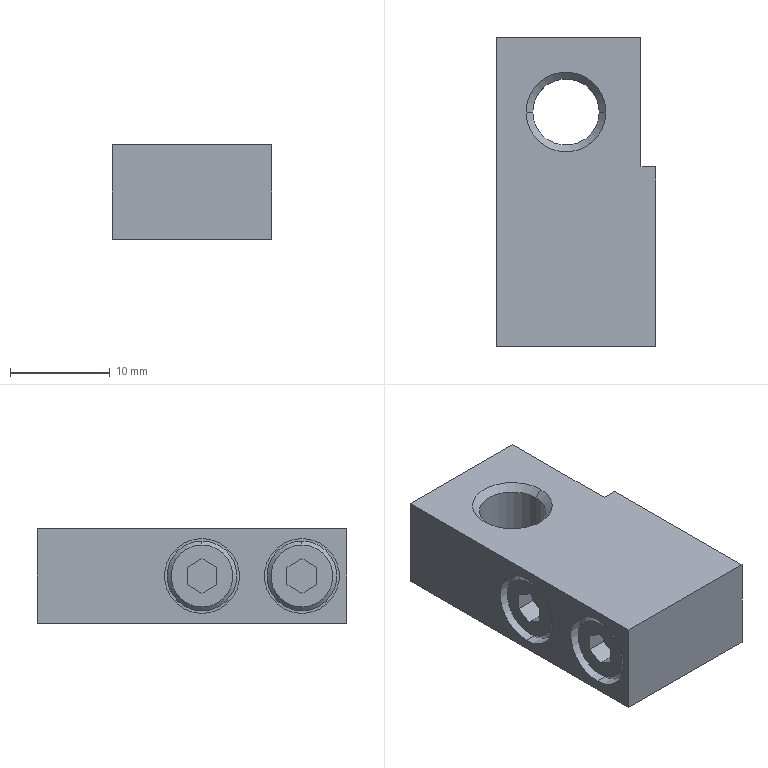Part | SolidWorks | features BaseBody 1 | 1 solid | 44 faces | box 16 x 31 x 9.5 mm | volume 4071 mm3 | plane 26 | cylinder 10 | cone 8 | commonest cylinder face diameters 7 x4 7.5 x4 6.647 x2
STEP:
#1=CARTESIAN_POINT('',(-15.6,4.5,3.1));
#2=VERTEX_POINT('',#1);
#3=CARTESIAN_POINT('',(-15.6,4.5,-3.1));
#4=VERTEX_POINT('',#3);
#5=CARTESIAN_POINT('',(-15.6,4.5,0.));
#6=DIRECTION('',(-1.,0.,0.));
#7=DIRECTION('',(0.,0.,1.));
#8=AXIS2_PLACEMENT_3D('',#5,#6,#7);
#9=CIRCLE('',#8,3.1);
#10=EDGE_CURVE('',#2,#4,#9,.T.);
#11=ORIENTED_EDGE('',*,*,#10,.F.);
#12=CARTESIAN_POINT('',(-15.2,4.5,3.5));
#13=VERTEX_POINT('',#12);
#14=CARTESIAN_POINT('',(-15.2,4.5,3.5));
#15=DIRECTION('',(0.7071,0.,0.7071));
#16=VECTOR('',#15,1000.);
#17=LINE('',#14,#16);
#18=EDGE_CURVE('',#2,#13,#17,.T.);
#19=ORIENTED_EDGE('',*,*,#18,.T.);
#20=CARTESIAN_POINT('',(-15.2,4.5,-3.5));
#21=VERTEX_POINT('',#20);
#22=CARTESIAN_POINT('',(-15.2,4.5,0.));
#23=DIRECTION('',(-1.,0.,0.));
#24=DIRECTION('',(0.,0.,1.));
#25=AXIS2_PLACEMENT_3D('',#22,#23,#24);
#26=CIRCLE('',#25,3.5);
#27=EDGE_CURVE('',#13,#21,#26,.T.);
#28=ORIENTED_EDGE('',*,*,#27,.T.);
#29=CARTESIAN_POINT('',(-15.2,4.5,-3.5));
#30=DIRECTION('',(0.7071,0.,-0.7071));
#31=VECTOR('',#30,1000.);
#32=LINE('',#29,#31);
#33=EDGE_CURVE('',#4,#21,#32,.T.);
#34=ORIENTED_EDGE('',*,*,#33,.F.);
#35=EDGE_LOOP('',(#11,#19,#28,#34));
#36=FACE_OUTER_BOUND('',#35,.T.);
#37=CARTESIAN_POINT('',(-15.2,4.5,0.));
#38=DIRECTION('',(1.,0.,0.));
#39=DIRECTION('',(0.,0.,-1.));
#40=AXIS2_PLACEMENT_3D('',#37,#38,#39);
#41=CONICAL_SURFACE('',#40,3.5,0.7854);
#42=ADVANCED_FACE('',(#36),#41,.T.);
#43=CARTESIAN_POINT('',(-5.677,23.5,4.074));
#44=VERTEX_POINT('',#43);
#45=CARTESIAN_POINT('',(-12.324,23.5,4.074));
#46=VERTEX_POINT('',#45);
#47=CARTESIAN_POINT('',(-9.,23.5,4.074));
#48=DIRECTION('',(0.,0.,-1.));
#49=DIRECTION('',(-1.,0.,0.));
#50=AXIS2_PLACEMENT_3D('',#47,#48,#49);
#51=CIRCLE('',#50,3.324);
#52=EDGE_CURVE('',#44,#46,#51,.T.);
#53=ORIENTED_EDGE('',*,*,#52,.F.);
#54=CARTESIAN_POINT('',(-5.677,23.5,-4.074));
#55=VERTEX_POINT('',#54);
#56=CARTESIAN_POINT('',(-5.677,23.5,-4.75));
#57=DIRECTION('',(0.,0.,-1.));
#58=VECTOR('',#57,1000.);
#59=LINE('',#56,#58);
#60=EDGE_CURVE('',#44,#55,#59,.T.);
#61=ORIENTED_EDGE('',*,*,#60,.T.);
#62=CARTESIAN_POINT('',(-12.324,23.5,-4.074));
#63=VERTEX_POINT('',#62);
#64=CARTESIAN_POINT('',(-9.,23.5,-4.074));
#65=DIRECTION('',(0.,0.,-1.));
#66=DIRECTION('',(-1.,0.,0.));
#67=AXIS2_PLACEMENT_3D('',#64,#65,#66);
#68=CIRCLE('',#67,3.324);
#69=EDGE_CURVE('',#55,#63,#68,.T.);
#70=ORIENTED_EDGE('',*,*,#69,.T.);
#71=CARTESIAN_POINT('',(-12.324,23.5,-4.75));
#72=DIRECTION('',(0.,0.,-1.));
#73=VECTOR('',#72,1000.);
#74=LINE('',#71,#73);
#75=EDGE_CURVE('',#46,#63,#74,.T.);
#76=ORIENTED_EDGE('',*,*,#75,.F.);
#77=EDGE_LOOP('',(#53,#61,#70,#76));
#78=FACE_OUTER_BOUND('',#77,.T.);
#79=CARTESIAN_POINT('',(-9.,23.5,-4.75));
#80=DIRECTION('',(0.,0.,-1.));
#81=DIRECTION('',(-1.,0.,0.));
#82=AXIS2_PLACEMENT_3D('',#79,#80,#81);
#83=CYLINDRICAL_SURFACE('',#82,3.324);
#84=ADVANCED_FACE('',(#78),#83,.F.);
#85=CARTESIAN_POINT('',(-11.6,4.5,3.5));
#86=VERTEX_POINT('',#85);
#87=CARTESIAN_POINT('',(-11.6,4.5,-3.5));
#88=VERTEX_POINT('',#87);
#89=CARTESIAN_POINT('',(-11.6,4.5,0.));
#90=DIRECTION('',(-1.,0.,0.));
#91=DIRECTION('',(0.,0.,-1.));
#92=AXIS2_PLACEMENT_3D('',#89,#90,#91);
#93=CIRCLE('',#92,3.5);
#94=EDGE_CURVE('',#86,#88,#93,.T.);
#95=ORIENTED_EDGE('',*,*,#94,.T.);
#96=CARTESIAN_POINT('',(-15.6,4.5,-3.5));
#97=DIRECTION('',(-1.,0.,0.));
#98=VECTOR('',#97,1000.);
#99=LINE('',#96,#98);
#100=EDGE_CURVE('',#88,#21,#99,.T.);
#101=ORIENTED_EDGE('',*,*,#100,.T.);
#102=ORIENTED_EDGE('',*,*,#27,.F.);
#103=CARTESIAN_POINT('',(-15.6,4.5,3.5));
#104=DIRECTION('',(-1.,0.,0.));
#105=VECTOR('',#104,1000.);
#106=LINE('',#103,#105);
#107=EDGE_CURVE('',#86,#13,#106,.T.);
#108=ORIENTED_EDGE('',*,*,#107,.F.);
#109=EDGE_LOOP('',(#95,#101,#102,#108));
#110=FACE_OUTER_BOUND('',#109,.T.);
#111=CARTESIAN_POINT('',(-15.6,4.5,0.));
#112=DIRECTION('',(-1.,0.,0.));
#113=DIRECTION('',(0.,0.,1.));
#114=AXIS2_PLACEMENT_3D('',#111,#112,#113);
#115=CYLINDRICAL_SURFACE('',#114,3.5);
#116=ADVANCED_FACE('',(#110),#115,.T.);
#117=ORIENTED_EDGE('',*,*,#52,.T.);
#118=CARTESIAN_POINT('',(-13.,23.5,4.75));
#119=VERTEX_POINT('',#118);
#120=CARTESIAN_POINT('',(-13.,23.5,4.75));
#121=DIRECTION('',(-0.7071,0.,0.7071));
#122=VECTOR('',#121,1000.);
#123=LINE('',#120,#122);
#124=EDGE_CURVE('',#46,#119,#123,.T.);
#125=ORIENTED_EDGE('',*,*,#124,.T.);
#126=CARTESIAN_POINT('',(-5.,23.5,4.75));
#127=VERTEX_POINT('',#126);
#128=CARTESIAN_POINT('',(-9.,23.5,4.75));
#129=DIRECTION('',(0.,0.,-1.));
#130=DIRECTION('',(-1.,0.,0.));
#131=AXIS2_PLACEMENT_3D('',#128,#129,#130);
#132=CIRCLE('',#131,4.);
#133=EDGE_CURVE('',#127,#119,#132,.T.);
#134=ORIENTED_EDGE('',*,*,#133,.F.);
#135=CARTESIAN_POINT('',(-5.,23.5,4.75));
#136=DIRECTION('',(0.7071,0.,0.7071));
#137=VECTOR('',#136,1000.);
#138=LINE('',#135,#137);
#139=EDGE_CURVE('',#44,#127,#138,.T.);
#140=ORIENTED_EDGE('',*,*,#139,.F.);
#141=EDGE_LOOP('',(#117,#125,#134,#140));
#142=FACE_OUTER_BOUND('',#141,.T.);
#143=CARTESIAN_POINT('',(-9.,23.5,4.75));
#144=DIRECTION('',(0.,0.,1.));
#145=DIRECTION('',(1.,0.,0.));
#146=AXIS2_PLACEMENT_3D('',#143,#144,#145);
#147=CONICAL_SURFACE('',#146,4.,0.7854);
#148=ADVANCED_FACE('',(#142),#147,.F.);
#149=ORIENTED_EDGE('',*,*,#69,.F.);
#150=CARTESIAN_POINT('',(-5.,23.5,-4.75));
#151=VERTEX_POINT('',#150);
#152=CARTESIAN_POINT('',(-5.677,23.5,-4.074));
#153=DIRECTION('',(0.7071,0.,-0.7071));
#154=VECTOR('',#153,1000.);
#155=LINE('',#152,#154);
#156=EDGE_CURVE('',#55,#151,#155,.T.);
#157=ORIENTED_EDGE('',*,*,#156,.T.);
#158=CARTESIAN_POINT('',(-13.,23.5,-4.75));
#159=VERTEX_POINT('',#158);
#160=CARTESIAN_POINT('',(-9.,23.5,-4.75));
#161=DIRECTION('',(0.,0.,-1.));
#162=DIRECTION('',(-1.,0.,0.));
#163=AXIS2_PLACEMENT_3D('',#160,#161,#162);
#164=CIRCLE('',#163,4.);
#165=EDGE_CURVE('',#151,#159,#164,.T.);
#166=ORIENTED_EDGE('',*,*,#165,.T.);
#167=CARTESIAN_POINT('',(-12.324,23.5,-4.074));
#168=DIRECTION('',(-0.7071,0.,-0.7071));
#169=VECTOR('',#168,1000.);
#170=LINE('',#167,#169);
#171=EDGE_CURVE('',#63,#159,#170,.T.);
#172=ORIENTED_EDGE('',*,*,#171,.F.);
#173=EDGE_LOOP('',(#149,#157,#166,#172));
#174=FACE_OUTER_BOUND('',#173,.T.);
#175=CARTESIAN_POINT('',(-9.,23.5,-4.074));
#176=DIRECTION('',(0.,0.,-1.));
#177=DIRECTION('',(-1.,0.,0.));
#178=AXIS2_PLACEMENT_3D('',#175,#176,#177);
#179=CONICAL_SURFACE('',#178,3.324,0.7854);
#180=ADVANCED_FACE('',(#174),#179,.F.);
#181=CARTESIAN_POINT('',(-11.6,4.5,3.75));
#182=VERTEX_POINT('',#181);
#183=CARTESIAN_POINT('',(-11.6,4.5,-3.75));
#184=VERTEX_POINT('',#183);
#185=CARTESIAN_POINT('',(-11.6,4.5,0.));
#186=DIRECTION('',(1.,0.,0.));
#187=DIRECTION('',(0.,0.,-1.));
#188=AXIS2_PLACEMENT_3D('',#185,#186,#187);
#189=CIRCLE('',#188,3.75);
#190=EDGE_CURVE('',#182,#184,#189,.T.);
#191=ORIENTED_EDGE('',*,*,#190,.T.);
#192=CARTESIAN_POINT('',(-16.,4.5,-3.75));
#193=VERTEX_POINT('',#192);
#194=CARTESIAN_POINT('',(-11.6,4.5,-3.75));
#195=DIRECTION('',(-1.,0.,0.));
#196=VECTOR('',#195,1000.);
#197=LINE('',#194,#196);
#198=EDGE_CURVE('',#184,#193,#197,.T.);
#199=ORIENTED_EDGE('',*,*,#198,.T.);
#200=CARTESIAN_POINT('',(-16.,4.5,3.75));
#201=VERTEX_POINT('',#200);
#202=CARTESIAN_POINT('',(-16.,4.5,0.));
#203=DIRECTION('',(1.,0.,0.));
#204=DIRECTION('',(0.,0.,-1.));
#205=AXIS2_PLACEMENT_3D('',#202,#203,#204);
#206=CIRCLE('',#205,3.75);
#207=EDGE_CURVE('',#201,#193,#206,.T.);
#208=ORIENTED_EDGE('',*,*,#207,.F.);
#209=CARTESIAN_POINT('',(-11.6,4.5,3.75));
#210=DIRECTION('',(-1.,0.,0.));
#211=VECTOR('',#210,1000.);
#212=LINE('',#209,#211);
#213=EDGE_CURVE('',#182,#201,#212,.T.);
#214=ORIENTED_EDGE('',*,*,#213,.F.);
#215=EDGE_LOOP('',(#191,#199,#208,#214));
#216=FACE_OUTER_BOUND('',#215,.T.);
#217=CARTESIAN_POINT('',(-11.6,4.5,0.));
#218=DIRECTION('',(-1.,0.,0.));
#219=DIRECTION('',(0.,0.,1.));
#220=AXIS2_PLACEMENT_3D('',#217,#218,#219);
#221=CYLINDRICAL_SURFACE('',#220,3.75);
#222=ADVANCED_FACE('',(#216),#221,.F.);
#223=CARTESIAN_POINT('',(-11.6,14.5,3.75));
#224=VERTEX_POINT('',#223);
#225=CARTESIAN_POINT('',(-11.6,14.5,-3.75));
#226=VERTEX_POINT('',#225);
#227=CARTESIAN_POINT('',(-11.6,14.5,0.));
#228=DIRECTION('',(1.,0.,0.));
#229=DIRECTION('',(0.,0.,-1.));
#230=AXIS2_PLACEMENT_3D('',#227,#228,#229);
#231=CIRCLE('',#230,3.75);
#232=EDGE_CURVE('',#224,#226,#231,.T.);
#233=ORIENTED_EDGE('',*,*,#232,.T.);
#234=CARTESIAN_POINT('',(-16.,14.5,-3.75));
#235=VERTEX_POINT('',#234);
#236=CARTESIAN_POINT('',(-11.6,14.5,-3.75));
#237=DIRECTION('',(-1.,0.,0.));
#238=VECTOR('',#237,1000.);
#239=LINE('',#236,#238);
#240=EDGE_CURVE('',#226,#235,#239,.T.);
#241=ORIENTED_EDGE('',*,*,#240,.T.);
#242=CARTESIAN_POINT('',(-16.,14.5,3.75));
#243=VERTEX_POINT('',#242);
#244=CARTESIAN_POINT('',(-16.,14.5,0.));
#245=DIRECTION('',(1.,0.,0.));
#246=DIRECTION('',(0.,0.,-1.));
#247=AXIS2_PLACEMENT_3D('',#244,#245,#246);
#248=CIRCLE('',#247,3.75);
#249=EDGE_CURVE('',#243,#235,#248,.T.);
#250=ORIENTED_EDGE('',*,*,#249,.F.);
#251=CARTESIAN_POINT('',(-11.6,14.5,3.75));
#252=DIRECTION('',(-1.,0.,0.));
#253=VECTOR('',#252,1000.);
#254=LINE('',#251,#253);
#255=EDGE_CURVE('',#224,#243,#254,.T.);
#256=ORIENTED_EDGE('',*,*,#255,.F.);
#257=EDGE_LOOP('',(#233,#241,#250,#256));
#258=FACE_OUTER_BOUND('',#257,.T.);
#259=CARTESIAN_POINT('',(-11.6,14.5,0.));
#260=DIRECTION('',(-1.,0.,0.));
#261=DIRECTION('',(0.,0.,1.));
#262=AXIS2_PLACEMENT_3D('',#259,#260,#261);
#263=CYLINDRICAL_SURFACE('',#262,3.75);
#264=ADVANCED_FACE('',(#258),#263,.F.);
#265=CARTESIAN_POINT('',(-11.6,14.5,3.5));
#266=VERTEX_POINT('',#265);
#267=CARTESIAN_POINT('',(-11.6,14.5,-3.5));
#268=VERTEX_POINT('',#267);
#269=CARTESIAN_POINT('',(-11.6,14.5,0.));
#270=DIRECTION('',(-1.,0.,0.));
#271=DIRECTION('',(0.,0.,-1.));
#272=AXIS2_PLACEMENT_3D('',#269,#270,#271);
#273=CIRCLE('',#272,3.5);
#274=EDGE_CURVE('',#266,#268,#273,.T.);
#275=ORIENTED_EDGE('',*,*,#274,.T.);
#276=CARTESIAN_POINT('',(-15.2,14.5,-3.5));
#277=VERTEX_POINT('',#276);
#278=CARTESIAN_POINT('',(-15.6,14.5,-3.5));
#279=DIRECTION('',(-1.,0.,0.));
#280=VECTOR('',#279,1000.);
#281=LINE('',#278,#280);
#282=EDGE_CURVE('',#268,#277,#281,.T.);
#283=ORIENTED_EDGE('',*,*,#282,.T.);
#284=CARTESIAN_POINT('',(-15.2,14.5,3.5));
#285=VERTEX_POINT('',#284);
#286=CARTESIAN_POINT('',(-15.2,14.5,0.));
#287=DIRECTION('',(-1.,0.,0.));
#288=DIRECTION('',(0.,0.,1.));
#289=AXIS2_PLACEMENT_3D('',#286,#287,#288);
#290=CIRCLE('',#289,3.5);
#291=EDGE_CURVE('',#285,#277,#290,.T.);
#292=ORIENTED_EDGE('',*,*,#291,.F.);
#293=CARTESIAN_POINT('',(-15.6,14.5,3.5));
#294=DIRECTION('',(-1.,0.,0.));
#295=VECTOR('',#294,1000.);
#296=LINE('',#293,#295);
#297=EDGE_CURVE('',#266,#285,#296,.T.);
#298=ORIENTED_EDGE('',*,*,#297,.F.);
#299=EDGE_LOOP('',(#275,#283,#292,#298));
#300=FACE_OUTER_BOUND('',#299,.T.);
#301=CARTESIAN_POINT('',(-15.6,14.5,0.));
#302=DIRECTION('',(-1.,0.,0.));
#303=DIRECTION('',(0.,0.,1.));
#304=AXIS2_PLACEMENT_3D('',#301,#302,#303);
#305=CYLINDRICAL_SURFACE('',#304,3.5);
#306=ADVANCED_FACE('',(#300),#305,.T.);
#307=CARTESIAN_POINT('',(-15.6,14.5,3.1));
#308=VERTEX_POINT('',#307);
#309=CARTESIAN_POINT('',(-15.6,14.5,-3.1));
#310=VERTEX_POINT('',#309);
#311=CARTESIAN_POINT('',(-15.6,14.5,0.));
#312=DIRECTION('',(-1.,0.,0.));
#313=DIRECTION('',(0.,0.,1.));
#314=AXIS2_PLACEMENT_3D('',#311,#312,#313);
#315=CIRCLE('',#314,3.1);
#316=EDGE_CURVE('',#308,#310,#315,.T.);
#317=ORIENTED_EDGE('',*,*,#316,.F.);
#318=CARTESIAN_POINT('',(-15.2,14.5,3.5));
#319=DIRECTION('',(0.7071,0.,0.7071));
#320=VECTOR('',#319,1000.);
#321=LINE('',#318,#320);
#322=EDGE_CURVE('',#308,#285,#321,.T.);
#323=ORIENTED_EDGE('',*,*,#322,.T.);
#324=ORIENTED_EDGE('',*,*,#291,.T.);
#325=CARTESIAN_POINT('',(-15.2,14.5,-3.5));
#326=DIRECTION('',(0.7071,0.,-0.7071));
#327=VECTOR('',#326,1000.);
#328=LINE('',#325,#327);
#329=EDGE_CURVE('',#310,#277,#328,.T.);
#330=ORIENTED_EDGE('',*,*,#329,.F.);
#331=EDGE_LOOP('',(#317,#323,#324,#330));
#332=FACE_OUTER_BOUND('',#331,.T.);
#333=CARTESIAN_POINT('',(-15.2,14.5,0.));
#334=DIRECTION('',(1.,0.,0.));
#335=DIRECTION('',(0.,0.,-1.));
#336=AXIS2_PLACEMENT_3D('',#333,#334,#335);
#337=CONICAL_SURFACE('',#336,3.5,0.7854);
#338=ADVANCED_FACE('',(#332),#337,.T.);
#339=CARTESIAN_POINT('',(-15.6,14.5,1.732));
#340=VERTEX_POINT('',#339);
#341=CARTESIAN_POINT('',(-15.6,13.,0.866));
#342=VERTEX_POINT('',#341);
#343=CARTESIAN_POINT('',(-15.6,14.5,1.732));
#344=DIRECTION('',(0.,-0.866,-0.5));
#345=VECTOR('',#344,1000.);
#346=LINE('',#343,#345);
#347=EDGE_CURVE('',#340,#342,#346,.T.);
#348=ORIENTED_EDGE('',*,*,#347,.T.);
#349=CARTESIAN_POINT('',(-15.6,13.,-0.866));
#350=VERTEX_POINT('',#349);
#351=CARTESIAN_POINT('',(-15.6,13.,-0.866));
#352=DIRECTION('',(0.,0.,1.));
#353=VECTOR('',#352,1000.);
#354=LINE('',#351,#353);
#355=EDGE_CURVE('',#350,#342,#354,.T.);
#356=ORIENTED_EDGE('',*,*,#355,.F.);
#357=CARTESIAN_POINT('',(-15.6,14.5,-1.732));
#358=VERTEX_POINT('',#357);
#359=CARTESIAN_POINT('',(-15.6,13.,-0.866));
#360=DIRECTION('',(0.,0.866,-0.5));
#361=VECTOR('',#360,1000.);
#362=LINE('',#359,#361);
#363=EDGE_CURVE('',#350,#358,#362,.T.);
#364=ORIENTED_EDGE('',*,*,#363,.T.);
#365=CARTESIAN_POINT('',(-15.6,16.,-0.866));
#366=VERTEX_POINT('',#365);
#367=CARTESIAN_POINT('',(-15.6,14.5,-1.732));
#368=DIRECTION('',(0.,0.866,0.5));
#369=VECTOR('',#368,1000.);
#370=LINE('',#367,#369);
#371=EDGE_CURVE('',#358,#366,#370,.T.);
#372=ORIENTED_EDGE('',*,*,#371,.T.);
#373=CARTESIAN_POINT('',(-15.6,16.,0.866));
#374=VERTEX_POINT('',#373);
#375=CARTESIAN_POINT('',(-15.6,16.,-0.866));
#376=DIRECTION('',(0.,0.,1.));
#377=VECTOR('',#376,1000.);
#378=LINE('',#375,#377);
#379=EDGE_CURVE('',#366,#374,#378,.T.);
#380=ORIENTED_EDGE('',*,*,#379,.T.);
#381=CARTESIAN_POINT('',(-15.6,16.,0.866));
#382=DIRECTION('',(0.,-0.866,0.5));
#383=VECTOR('',#382,1000.);
#384=LINE('',#381,#383);
#385=EDGE_CURVE('',#374,#340,#384,.T.);
#386=ORIENTED_EDGE('',*,*,#385,.T.);
#387=EDGE_LOOP('',(#348,#356,#364,#372,#380,#386));
#388=FACE_BOUND('',#387,.T.);
#389=CARTESIAN_POINT('',(-15.6,14.5,0.));
#390=DIRECTION('',(-1.,0.,0.));
#391=DIRECTION('',(0.,0.,1.));
#392=AXIS2_PLACEMENT_3D('',#389,#390,#391);
#393=CIRCLE('',#392,3.1);
#394=EDGE_CURVE('',#310,#308,#393,.T.);
#395=ORIENTED_EDGE('',*,*,#394,.T.);
#396=ORIENTED_EDGE('',*,*,#316,.T.);
#397=EDGE_LOOP('',(#395,#396));
#398=FACE_OUTER_BOUND('',#397,.T.);
#399=CARTESIAN_POINT('',(-15.6,11.4,0.));
#400=DIRECTION('',(1.,0.,0.));
#401=DIRECTION('',(0.,0.,-1.));
#402=AXIS2_PLACEMENT_3D('',#399,#400,#401);
#403=PLANE('',#402);
#404=ADVANCED_FACE('',(#388,#398),#403,.F.);
#405=ORIENTED_EDGE('',*,*,#347,.F.);
#406=CARTESIAN_POINT('',(-13.6,14.5,1.732));
#407=VERTEX_POINT('',#406);
#408=CARTESIAN_POINT('',(-13.6,14.5,1.732));
#409=DIRECTION('',(-1.,0.,0.));
#410=VECTOR('',#409,1000.);
#411=LINE('',#408,#410);
#412=EDGE_CURVE('',#407,#340,#411,.T.);
#413=ORIENTED_EDGE('',*,*,#412,.F.);
#414=CARTESIAN_POINT('',(-13.6,13.,0.866));
#415=VERTEX_POINT('',#414);
#416=CARTESIAN_POINT('',(-13.6,14.5,1.732));
#417=DIRECTION('',(0.,-0.866,-0.5));
#418=VECTOR('',#417,1000.);
#419=LINE('',#416,#418);
#420=EDGE_CURVE('',#407,#415,#419,.T.);
#421=ORIENTED_EDGE('',*,*,#420,.T.);
#422=CARTESIAN_POINT('',(-13.6,13.,0.866));
#423=DIRECTION('',(-1.,0.,0.));
#424=VECTOR('',#423,1000.);
#425=LINE('',#422,#424);
#426=EDGE_CURVE('',#415,#342,#425,.T.);
#427=ORIENTED_EDGE('',*,*,#426,.T.);
#428=EDGE_LOOP('',(#405,#413,#421,#427));
#429=FACE_OUTER_BOUND('',#428,.T.);
#430=CARTESIAN_POINT('',(-13.6,14.5,1.732));
#431=DIRECTION('',(0.,0.5,-0.866));
#432=DIRECTION('',(0.,0.866,0.5));
#433=AXIS2_PLACEMENT_3D('',#430,#431,#432);
#434=PLANE('',#433);
#435=ADVANCED_FACE('',(#429),#434,.T.);
#436=ORIENTED_EDGE('',*,*,#355,.T.);
#437=ORIENTED_EDGE('',*,*,#426,.F.);
#438=CARTESIAN_POINT('',(-13.6,13.,-0.866));
#439=VERTEX_POINT('',#438);
#440=CARTESIAN_POINT('',(-13.6,13.,0.866));
#441=DIRECTION('',(0.,0.,-1.));
#442=VECTOR('',#441,1000.);
#443=LINE('',#440,#442);
#444=EDGE_CURVE('',#415,#439,#443,.T.);
#445=ORIENTED_EDGE('',*,*,#444,.T.);
#446=CARTESIAN_POINT('',(-13.6,13.,-0.866));
#447=DIRECTION('',(-1.,0.,0.));
#448=VECTOR('',#447,1000.);
#449=LINE('',#446,#448);
#450=EDGE_CURVE('',#439,#350,#449,.T.);
#451=ORIENTED_EDGE('',*,*,#450,.T.);
#452=EDGE_LOOP('',(#436,#437,#445,#451));
#453=FACE_OUTER_BOUND('',#452,.T.);
#454=CARTESIAN_POINT('',(-13.6,13.,0.866));
#455=DIRECTION('',(0.,1.,0.));
#456=DIRECTION('',(0.,0.,1.));
#457=AXIS2_PLACEMENT_3D('',#454,#455,#456);
#458=PLANE('',#457);
#459=ADVANCED_FACE('',(#453),#458,.T.);
#460=ORIENTED_EDGE('',*,*,#363,.F.);
#461=ORIENTED_EDGE('',*,*,#450,.F.);
#462=CARTESIAN_POINT('',(-13.6,14.5,-1.732));
#463=VERTEX_POINT('',#462);
#464=CARTESIAN_POINT('',(-13.6,13.,-0.866));
#465=DIRECTION('',(0.,0.866,-0.5));
#466=VECTOR('',#465,1000.);
#467=LINE('',#464,#466);
#468=EDGE_CURVE('',#439,#463,#467,.T.);
#469=ORIENTED_EDGE('',*,*,#468,.T.);
#470=CARTESIAN_POINT('',(-13.6,14.5,-1.732));
#471=DIRECTION('',(-1.,0.,0.));
#472=VECTOR('',#471,1000.);
#473=LINE('',#470,#472);
#474=EDGE_CURVE('',#463,#358,#473,.T.);
#475=ORIENTED_EDGE('',*,*,#474,.T.);
#476=EDGE_LOOP('',(#460,#461,#469,#475));
#477=FACE_OUTER_BOUND('',#476,.T.);
#478=CARTESIAN_POINT('',(-13.6,13.,-0.866));
#479=DIRECTION('',(0.,0.5,0.866));
#480=DIRECTION('',(0.,-0.866,0.5));
#481=AXIS2_PLACEMENT_3D('',#478,#479,#480);
#482=PLANE('',#481);
#483=ADVANCED_FACE('',(#477),#482,.T.);
#484=ORIENTED_EDGE('',*,*,#371,.F.);
#485=ORIENTED_EDGE('',*,*,#474,.F.);
#486=CARTESIAN_POINT('',(-13.6,16.,-0.866));
#487=VERTEX_POINT('',#486);
#488=CARTESIAN_POINT('',(-13.6,14.5,-1.732));
#489=DIRECTION('',(0.,0.866,0.5));
#490=VECTOR('',#489,1000.);
#491=LINE('',#488,#490);
#492=EDGE_CURVE('',#463,#487,#491,.T.);
#493=ORIENTED_EDGE('',*,*,#492,.T.);
#494=CARTESIAN_POINT('',(-13.6,16.,-0.866));
#495=DIRECTION('',(-1.,0.,0.));
#496=VECTOR('',#495,1000.);
#497=LINE('',#494,#496);
#498=EDGE_CURVE('',#487,#366,#497,.T.);
#499=ORIENTED_EDGE('',*,*,#498,.T.);
#500=EDGE_LOOP('',(#484,#485,#493,#499));
#501=FACE_OUTER_BOUND('',#500,.T.);
#502=CARTESIAN_POINT('',(-13.6,14.5,-1.732));
#503=DIRECTION('',(0.,-0.5,0.866));
#504=DIRECTION('',(0.,-0.866,-0.5));
#505=AXIS2_PLACEMENT_3D('',#502,#503,#504);
#506=PLANE('',#505);
#507=ADVANCED_FACE('',(#501),#506,.T.);
#508=ORIENTED_EDGE('',*,*,#379,.F.);
#509=ORIENTED_EDGE('',*,*,#498,.F.);
#510=CARTESIAN_POINT('',(-13.6,16.,0.866));
#511=VERTEX_POINT('',#510);
#512=CARTESIAN_POINT('',(-13.6,16.,-0.866));
#513=DIRECTION('',(0.,0.,1.));
#514=VECTOR('',#513,1000.);
#515=LINE('',#512,#514);
#516=EDGE_CURVE('',#487,#511,#515,.T.);
#517=ORIENTED_EDGE('',*,*,#516,.T.);
#518=CARTESIAN_POINT('',(-13.6,16.,0.866));
#519=DIRECTION('',(-1.,0.,0.));
#520=VECTOR('',#519,1000.);
#521=LINE('',#518,#520);
#522=EDGE_CURVE('',#511,#374,#521,.T.);
#523=ORIENTED_EDGE('',*,*,#522,.T.);
#524=EDGE_LOOP('',(#508,#509,#517,#523));
#525=FACE_OUTER_BOUND('',#524,.T.);
#526=CARTESIAN_POINT('',(-13.6,16.,-0.866));
#527=DIRECTION('',(0.,-1.,0.));
#528=DIRECTION('',(0.,0.,-1.));
#529=AXIS2_PLACEMENT_3D('',#526,#527,#528);
#530=PLANE('',#529);
#531=ADVANCED_FACE('',(#525),#530,.T.);
#532=ORIENTED_EDGE('',*,*,#385,.F.);
#533=ORIENTED_EDGE('',*,*,#522,.F.);
#534=CARTESIAN_POINT('',(-13.6,16.,0.866));
#535=DIRECTION('',(0.,-0.866,0.5));
#536=VECTOR('',#535,1000.);
#537=LINE('',#534,#536);
#538=EDGE_CURVE('',#511,#407,#537,.T.);
#539=ORIENTED_EDGE('',*,*,#538,.T.);
#540=ORIENTED_EDGE('',*,*,#412,.T.);
#541=EDGE_LOOP('',(#532,#533,#539,#540));
#542=FACE_OUTER_BOUND('',#541,.T.);
#543=CARTESIAN_POINT('',(-13.6,16.,0.866));
#544=DIRECTION('',(0.,-0.5,-0.866));
#545=DIRECTION('',(0.,0.866,-0.5));
#546=AXIS2_PLACEMENT_3D('',#543,#544,#545);
#547=PLANE('',#546);
#548=ADVANCED_FACE('',(#542),#547,.T.);
#549=ORIENTED_EDGE('',*,*,#322,.F.);
#550=ORIENTED_EDGE('',*,*,#394,.F.);
#551=ORIENTED_EDGE('',*,*,#329,.T.);
#552=CARTESIAN_POINT('',(-15.2,14.5,0.));
#553=DIRECTION('',(-1.,0.,0.));
#554=DIRECTION('',(0.,0.,1.));
#555=AXIS2_PLACEMENT_3D('',#552,#553,#554);
#556=CIRCLE('',#555,3.5);
#557=EDGE_CURVE('',#277,#285,#556,.T.);
#558=ORIENTED_EDGE('',*,*,#557,.T.);
#559=EDGE_LOOP('',(#549,#550,#551,#558));
#560=FACE_OUTER_BOUND('',#559,.T.);
#561=CARTESIAN_POINT('',(-15.2,14.5,0.));
#562=DIRECTION('',(1.,0.,0.));
#563=DIRECTION('',(0.,0.,-1.));
#564=AXIS2_PLACEMENT_3D('',#561,#562,#563);
#565=CONICAL_SURFACE('',#564,3.5,0.7854);
#566=ADVANCED_FACE('',(#560),#565,.T.);
#567=ORIENTED_EDGE('',*,*,#538,.F.);
#568=ORIENTED_EDGE('',*,*,#516,.F.);
#569=ORIENTED_EDGE('',*,*,#492,.F.);
#570=ORIENTED_EDGE('',*,*,#468,.F.);
#571=ORIENTED_EDGE('',*,*,#444,.F.);
#572=ORIENTED_EDGE('',*,*,#420,.F.);
#573=EDGE_LOOP('',(#567,#568,#569,#570,#571,#572));
#574=FACE_OUTER_BOUND('',#573,.T.);
#575=CARTESIAN_POINT('',(-13.6,10.,0.));
#576=DIRECTION('',(1.,0.,0.));
#577=DIRECTION('',(0.,0.,-1.));
#578=AXIS2_PLACEMENT_3D('',#575,#576,#577);
#579=PLANE('',#578);
#580=ADVANCED_FACE('',(#574),#579,.F.);
#581=ORIENTED_EDGE('',*,*,#282,.F.);
#582=CARTESIAN_POINT('',(-11.6,14.5,0.));
#583=DIRECTION('',(-1.,0.,0.));
#584=DIRECTION('',(0.,0.,-1.));
#585=AXIS2_PLACEMENT_3D('',#582,#583,#584);
#586=CIRCLE('',#585,3.5);
#587=EDGE_CURVE('',#268,#266,#586,.T.);
#588=ORIENTED_EDGE('',*,*,#587,.T.);
#589=ORIENTED_EDGE('',*,*,#297,.T.);
#590=ORIENTED_EDGE('',*,*,#557,.F.);
#591=EDGE_LOOP('',(#581,#588,#589,#590));
#592=FACE_OUTER_BOUND('',#591,.T.);
#593=CARTESIAN_POINT('',(-15.6,14.5,0.));
#594=DIRECTION('',(-1.,0.,0.));
#595=DIRECTION('',(0.,0.,1.));
#596=AXIS2_PLACEMENT_3D('',#593,#594,#595);
#597=CYLINDRICAL_SURFACE('',#596,3.5);
#598=ADVANCED_FACE('',(#592),#597,.T.);
#599=ORIENTED_EDGE('',*,*,#274,.F.);
#600=ORIENTED_EDGE('',*,*,#587,.F.);
#601=EDGE_LOOP('',(#599,#600));
#602=FACE_BOUND('',#601,.T.);
#603=ORIENTED_EDGE('',*,*,#232,.F.);
#604=CARTESIAN_POINT('',(-11.6,14.5,0.));
#605=DIRECTION('',(1.,0.,0.));
#606=DIRECTION('',(0.,0.,-1.));
#607=AXIS2_PLACEMENT_3D('',#604,#605,#606);
#608=CIRCLE('',#607,3.75);
#609=EDGE_CURVE('',#226,#224,#608,.T.);
#610=ORIENTED_EDGE('',*,*,#609,.F.);
#611=EDGE_LOOP('',(#603,#610));
#612=FACE_OUTER_BOUND('',#611,.T.);
#613=CARTESIAN_POINT('',(-11.6,14.5,0.));
#614=DIRECTION('',(1.,0.,0.));
#615=DIRECTION('',(0.,0.,-1.));
#616=AXIS2_PLACEMENT_3D('',#613,#614,#615);
#617=PLANE('',#616);
#618=ADVANCED_FACE('',(#602,#612),#617,.F.);
#619=ORIENTED_EDGE('',*,*,#240,.F.);
#620=ORIENTED_EDGE('',*,*,#609,.T.);
#621=ORIENTED_EDGE('',*,*,#255,.T.);
#622=CARTESIAN_POINT('',(-16.,14.5,0.));
#623=DIRECTION('',(1.,0.,0.));
#624=DIRECTION('',(0.,0.,-1.));
#625=AXIS2_PLACEMENT_3D('',#622,#623,#624);
#626=CIRCLE('',#625,3.75);
#627=EDGE_CURVE('',#235,#243,#626,.T.);
#628=ORIENTED_EDGE('',*,*,#627,.F.);
#629=EDGE_LOOP('',(#619,#620,#621,#628));
#630=FACE_OUTER_BOUND('',#629,.T.);
#631=CARTESIAN_POINT('',(-11.6,14.5,0.));
#632=DIRECTION('',(-1.,0.,0.));
#633=DIRECTION('',(0.,0.,1.));
#634=AXIS2_PLACEMENT_3D('',#631,#632,#633);
#635=CYLINDRICAL_SURFACE('',#634,3.75);
#636=ADVANCED_FACE('',(#630),#635,.F.);
#637=ORIENTED_EDGE('',*,*,#249,.T.);
#638=ORIENTED_EDGE('',*,*,#627,.T.);
#639=EDGE_LOOP('',(#637,#638));
#640=FACE_BOUND('',#639,.T.);
#641=ORIENTED_EDGE('',*,*,#207,.T.);
#642=CARTESIAN_POINT('',(-16.,4.5,0.));
#643=DIRECTION('',(1.,0.,0.));
#644=DIRECTION('',(0.,0.,-1.));
#645=AXIS2_PLACEMENT_3D('',#642,#643,#644);
#646=CIRCLE('',#645,3.75);
#647=EDGE_CURVE('',#193,#201,#646,.T.);
#648=ORIENTED_EDGE('',*,*,#647,.T.);
#649=EDGE_LOOP('',(#641,#648));
#650=FACE_BOUND('',#649,.T.);
#651=CARTESIAN_POINT('',(-16.,31.,-4.75));
#652=VERTEX_POINT('',#651);
#653=CARTESIAN_POINT('',(-16.,0.,-4.75));
#654=VERTEX_POINT('',#653);
#655=CARTESIAN_POINT('',(-16.,31.,-4.75));
#656=DIRECTION('',(0.,-1.,0.));
#657=VECTOR('',#656,1000.);
#658=LINE('',#655,#657);
#659=EDGE_CURVE('',#652,#654,#658,.T.);
#660=ORIENTED_EDGE('',*,*,#659,.T.);
#661=CARTESIAN_POINT('',(-16.,0.,4.75));
#662=VERTEX_POINT('',#661);
#663=CARTESIAN_POINT('',(-16.,0.,4.75));
#664=DIRECTION('',(0.,0.,-1.));
#665=VECTOR('',#664,1000.);
#666=LINE('',#663,#665);
#667=EDGE_CURVE('',#662,#654,#666,.T.);
#668=ORIENTED_EDGE('',*,*,#667,.F.);
#669=CARTESIAN_POINT('',(-16.,31.,4.75));
#670=VERTEX_POINT('',#669);
#671=CARTESIAN_POINT('',(-16.,31.,4.75));
#672=DIRECTION('',(0.,-1.,0.));
#673=VECTOR('',#672,1000.);
#674=LINE('',#671,#673);
#675=EDGE_CURVE('',#670,#662,#674,.T.);
#676=ORIENTED_EDGE('',*,*,#675,.F.);
#677=CARTESIAN_POINT('',(-16.,31.,4.75));
#678=DIRECTION('',(0.,0.,-1.));
#679=VECTOR('',#678,1000.);
#680=LINE('',#677,#679);
#681=EDGE_CURVE('',#670,#652,#680,.T.);
#682=ORIENTED_EDGE('',*,*,#681,.T.);
#683=EDGE_LOOP('',(#660,#668,#676,#682));
#684=FACE_OUTER_BOUND('',#683,.T.);
#685=CARTESIAN_POINT('',(-16.,31.,4.75));
#686=DIRECTION('',(1.,0.,0.));
#687=DIRECTION('',(0.,0.,-1.));
#688=AXIS2_PLACEMENT_3D('',#685,#686,#687);
#689=PLANE('',#688);
#690=ADVANCED_FACE('',(#640,#650,#684),#689,.F.);
#691=ORIENTED_EDGE('',*,*,#198,.F.);
#692=CARTESIAN_POINT('',(-11.6,4.5,0.));
#693=DIRECTION('',(1.,0.,0.));
#694=DIRECTION('',(0.,0.,-1.));
#695=AXIS2_PLACEMENT_3D('',#692,#693,#694);
#696=CIRCLE('',#695,3.75);
#697=EDGE_CURVE('',#184,#182,#696,.T.);
#698=ORIENTED_EDGE('',*,*,#697,.T.);
#699=ORIENTED_EDGE('',*,*,#213,.T.);
#700=ORIENTED_EDGE('',*,*,#647,.F.);
#701=EDGE_LOOP('',(#691,#698,#699,#700));
#702=FACE_OUTER_BOUND('',#701,.T.);
#703=CARTESIAN_POINT('',(-11.6,4.5,0.));
#704=DIRECTION('',(-1.,0.,0.));
#705=DIRECTION('',(0.,0.,1.));
#706=AXIS2_PLACEMENT_3D('',#703,#704,#705);
#707=CYLINDRICAL_SURFACE('',#706,3.75);
#708=ADVANCED_FACE('',(#702),#707,.F.);
#709=CARTESIAN_POINT('',(-9.,23.5,-4.75));
#710=DIRECTION('',(0.,0.,-1.));
#711=DIRECTION('',(-1.,0.,0.));
#712=AXIS2_PLACEMENT_3D('',#709,#710,#711);
#713=CIRCLE('',#712,4.);
#714=EDGE_CURVE('',#159,#151,#713,.T.);
#715=ORIENTED_EDGE('',*,*,#714,.F.);
#716=ORIENTED_EDGE('',*,*,#165,.F.);
#717=EDGE_LOOP('',(#715,#716));
#718=FACE_BOUND('',#717,.T.);
#719=CARTESIAN_POINT('',(-1.5,31.,-4.75));
#720=VERTEX_POINT('',#719);
#721=CARTESIAN_POINT('',(-1.5,31.,-4.75));
#722=DIRECTION('',(-1.,0.,0.));
#723=VECTOR('',#722,1000.);
#724=LINE('',#721,#723);
#725=EDGE_CURVE('',#720,#652,#724,.T.);
#726=ORIENTED_EDGE('',*,*,#725,.F.);
#727=CARTESIAN_POINT('',(-1.5,18.,-4.75));
#728=VERTEX_POINT('',#727);
#729=CARTESIAN_POINT('',(-1.5,18.,-4.75));
#730=DIRECTION('',(0.,1.,0.));
#731=VECTOR('',#730,1000.);
#732=LINE('',#729,#731);
#733=EDGE_CURVE('',#728,#720,#732,.T.);
#734=ORIENTED_EDGE('',*,*,#733,.F.);
#735=CARTESIAN_POINT('',(0.,18.,-4.75));
#736=VERTEX_POINT('',#735);
#737=CARTESIAN_POINT('',(0.,18.,-4.75));
#738=DIRECTION('',(-1.,0.,0.));
#739=VECTOR('',#738,1000.);
#740=LINE('',#737,#739);
#741=EDGE_CURVE('',#736,#728,#740,.T.);
#742=ORIENTED_EDGE('',*,*,#741,.F.);
#743=CARTESIAN_POINT('',(0.,0.,-4.75));
#744=VERTEX_POINT('',#743);
#745=CARTESIAN_POINT('',(0.,0.,-4.75));
#746=DIRECTION('',(0.,1.,0.));
#747=VECTOR('',#746,1000.);
#748=LINE('',#745,#747);
#749=EDGE_CURVE('',#744,#736,#748,.T.);
#750=ORIENTED_EDGE('',*,*,#749,.F.);
#751=CARTESIAN_POINT('',(-16.,0.,-4.75));
#752=DIRECTION('',(1.,0.,0.));
#753=VECTOR('',#752,1000.);
#754=LINE('',#751,#753);
#755=EDGE_CURVE('',#654,#744,#754,.T.);
#756=ORIENTED_EDGE('',*,*,#755,.F.);
#757=ORIENTED_EDGE('',*,*,#659,.F.);
#758=EDGE_LOOP('',(#726,#734,#742,#750,#756,#757));
#759=FACE_OUTER_BOUND('',#758,.T.);
#760=CARTESIAN_POINT('',(0.,0.,-4.75));
#761=DIRECTION('',(0.,0.,1.));
#762=DIRECTION('',(1.,0.,0.));
#763=AXIS2_PLACEMENT_3D('',#760,#761,#762);
#764=PLANE('',#763);
#765=ADVANCED_FACE('',(#718,#759),#764,.F.);
#766=ORIENTED_EDGE('',*,*,#755,.T.);
#767=CARTESIAN_POINT('',(0.,0.,4.75));
#768=VERTEX_POINT('',#767);
#769=CARTESIAN_POINT('',(0.,0.,4.75));
#770=DIRECTION('',(0.,0.,-1.));
#771=VECTOR('',#770,1000.);
#772=LINE('',#769,#771);
#773=EDGE_CURVE('',#768,#744,#772,.T.);
#774=ORIENTED_EDGE('',*,*,#773,.F.);
#775=CARTESIAN_POINT('',(-16.,0.,4.75));
#776=DIRECTION('',(1.,0.,0.));
#777=VECTOR('',#776,1000.);
#778=LINE('',#775,#777);
#779=EDGE_CURVE('',#662,#768,#778,.T.);
#780=ORIENTED_EDGE('',*,*,#779,.F.);
#781=ORIENTED_EDGE('',*,*,#667,.T.);
#782=EDGE_LOOP('',(#766,#774,#780,#781));
#783=FACE_OUTER_BOUND('',#782,.T.);
#784=CARTESIAN_POINT('',(-16.,0.,4.75));
#785=DIRECTION('',(0.,1.,0.));
#786=DIRECTION('',(0.,0.,1.));
#787=AXIS2_PLACEMENT_3D('',#784,#785,#786);
#788=PLANE('',#787);
#789=ADVANCED_FACE('',(#783),#788,.F.);
#790=ORIENTED_EDGE('',*,*,#133,.T.);
#791=CARTESIAN_POINT('',(-9.,23.5,4.75));
#792=DIRECTION('',(0.,0.,-1.));
#793=DIRECTION('',(-1.,0.,0.));
#794=AXIS2_PLACEMENT_3D('',#791,#792,#793);
#795=CIRCLE('',#794,4.);
#796=EDGE_CURVE('',#119,#127,#795,.T.);
#797=ORIENTED_EDGE('',*,*,#796,.T.);
#798=EDGE_LOOP('',(#790,#797));
#799=FACE_BOUND('',#798,.T.);
#800=CARTESIAN_POINT('',(-1.5,31.,4.75));
#801=VERTEX_POINT('',#800);
#802=CARTESIAN_POINT('',(-1.5,31.,4.75));
#803=DIRECTION('',(-1.,0.,0.));
#804=VECTOR('',#803,1000.);
#805=LINE('',#802,#804);
#806=EDGE_CURVE('',#801,#670,#805,.T.);
#807=ORIENTED_EDGE('',*,*,#806,.T.);
#808=ORIENTED_EDGE('',*,*,#675,.T.);
#809=ORIENTED_EDGE('',*,*,#779,.T.);
#810=CARTESIAN_POINT('',(0.,18.,4.75));
#811=VERTEX_POINT('',#810);
#812=CARTESIAN_POINT('',(0.,0.,4.75));
#813=DIRECTION('',(0.,1.,0.));
#814=VECTOR('',#813,1000.);
#815=LINE('',#812,#814);
#816=EDGE_CURVE('',#768,#811,#815,.T.);
#817=ORIENTED_EDGE('',*,*,#816,.T.);
#818=CARTESIAN_POINT('',(-1.5,18.,4.75));
#819=VERTEX_POINT('',#818);
#820=CARTESIAN_POINT('',(0.,18.,4.75));
#821=DIRECTION('',(-1.,0.,0.));
#822=VECTOR('',#821,1000.);
#823=LINE('',#820,#822);
#824=EDGE_CURVE('',#811,#819,#823,.T.);
#825=ORIENTED_EDGE('',*,*,#824,.T.);
#826=CARTESIAN_POINT('',(-1.5,18.,4.75));
#827=DIRECTION('',(0.,1.,0.));
#828=VECTOR('',#827,1000.);
#829=LINE('',#826,#828);
#830=EDGE_CURVE('',#819,#801,#829,.T.);
#831=ORIENTED_EDGE('',*,*,#830,.T.);
#832=EDGE_LOOP('',(#807,#808,#809,#817,#825,#831));
#833=FACE_OUTER_BOUND('',#832,.T.);
#834=CARTESIAN_POINT('',(0.,0.,4.75));
#835=DIRECTION('',(0.,0.,1.));
#836=DIRECTION('',(1.,0.,0.));
#837=AXIS2_PLACEMENT_3D('',#834,#835,#836);
#838=PLANE('',#837);
#839=ADVANCED_FACE('',(#799,#833),#838,.T.);
#840=ORIENTED_EDGE('',*,*,#725,.T.);
#841=ORIENTED_EDGE('',*,*,#681,.F.);
#842=ORIENTED_EDGE('',*,*,#806,.F.);
#843=CARTESIAN_POINT('',(-1.5,31.,4.75));
#844=DIRECTION('',(0.,0.,-1.));
#845=VECTOR('',#844,1000.);
#846=LINE('',#843,#845);
#847=EDGE_CURVE('',#801,#720,#846,.T.);
#848=ORIENTED_EDGE('',*,*,#847,.T.);
#849=EDGE_LOOP('',(#840,#841,#842,#848));
#850=FACE_OUTER_BOUND('',#849,.T.);
#851=CARTESIAN_POINT('',(-1.5,31.,4.75));
#852=DIRECTION('',(0.,-1.,0.));
#853=DIRECTION('',(0.,0.,-1.));
#854=AXIS2_PLACEMENT_3D('',#851,#852,#853);
#855=PLANE('',#854);
#856=ADVANCED_FACE('',(#850),#855,.F.);
#857=ORIENTED_EDGE('',*,*,#94,.F.);
#858=CARTESIAN_POINT('',(-11.6,4.5,0.));
#859=DIRECTION('',(-1.,0.,0.));
#860=DIRECTION('',(0.,0.,-1.));
#861=AXIS2_PLACEMENT_3D('',#858,#859,#860);
#862=CIRCLE('',#861,3.5);
#863=EDGE_CURVE('',#88,#86,#862,.T.);
#864=ORIENTED_EDGE('',*,*,#863,.F.);
#865=EDGE_LOOP('',(#857,#864));
#866=FACE_BOUND('',#865,.T.);
#867=ORIENTED_EDGE('',*,*,#190,.F.);
#868=ORIENTED_EDGE('',*,*,#697,.F.);
#869=EDGE_LOOP('',(#867,#868));
#870=FACE_OUTER_BOUND('',#869,.T.);
#871=CARTESIAN_POINT('',(-11.6,4.5,0.));
#872=DIRECTION('',(1.,0.,0.));
#873=DIRECTION('',(0.,0.,-1.));
#874=AXIS2_PLACEMENT_3D('',#871,#872,#873);
#875=PLANE('',#874);
#876=ADVANCED_FACE('',(#866,#870),#875,.F.);
#877=ORIENTED_EDGE('',*,*,#156,.F.);
#878=CARTESIAN_POINT('',(-9.,23.5,-4.074));
#879=DIRECTION('',(0.,0.,-1.));
#880=DIRECTION('',(-1.,0.,0.));
#881=AXIS2_PLACEMENT_3D('',#878,#879,#880);
#882=CIRCLE('',#881,3.324);
#883=EDGE_CURVE('',#63,#55,#882,.T.);
#884=ORIENTED_EDGE('',*,*,#883,.F.);
#885=ORIENTED_EDGE('',*,*,#171,.T.);
#886=ORIENTED_EDGE('',*,*,#714,.T.);
#887=EDGE_LOOP('',(#877,#884,#885,#886));
#888=FACE_OUTER_BOUND('',#887,.T.);
#889=CARTESIAN_POINT('',(-9.,23.5,-4.074));
#890=DIRECTION('',(0.,0.,-1.));
#891=DIRECTION('',(-1.,0.,0.));
#892=AXIS2_PLACEMENT_3D('',#889,#890,#891);
#893=CONICAL_SURFACE('',#892,3.324,0.7854);
#894=ADVANCED_FACE('',(#888),#893,.F.);
#895=ORIENTED_EDGE('',*,*,#733,.T.);
#896=ORIENTED_EDGE('',*,*,#847,.F.);
#897=ORIENTED_EDGE('',*,*,#830,.F.);
#898=CARTESIAN_POINT('',(-1.5,18.,4.75));
#899=DIRECTION('',(0.,0.,-1.));
#900=VECTOR('',#899,1000.);
#901=LINE('',#898,#900);
#902=EDGE_CURVE('',#819,#728,#901,.T.);
#903=ORIENTED_EDGE('',*,*,#902,.T.);
#904=EDGE_LOOP('',(#895,#896,#897,#903));
#905=FACE_OUTER_BOUND('',#904,.T.);
#906=CARTESIAN_POINT('',(-1.5,18.,4.75));
#907=DIRECTION('',(-1.,0.,0.));
#908=DIRECTION('',(0.,0.,1.));
#909=AXIS2_PLACEMENT_3D('',#906,#907,#908);
#910=PLANE('',#909);
#911=ADVANCED_FACE('',(#905),#910,.F.);
#912=ORIENTED_EDGE('',*,*,#741,.T.);
#913=ORIENTED_EDGE('',*,*,#902,.F.);
#914=ORIENTED_EDGE('',*,*,#824,.F.);
#915=CARTESIAN_POINT('',(0.,18.,4.75));
#916=DIRECTION('',(0.,0.,-1.));
#917=VECTOR('',#916,1000.);
#918=LINE('',#915,#917);
#919=EDGE_CURVE('',#811,#736,#918,.T.);
#920=ORIENTED_EDGE('',*,*,#919,.T.);
#921=EDGE_LOOP('',(#912,#913,#914,#920));
#922=FACE_OUTER_BOUND('',#921,.T.);
#923=CARTESIAN_POINT('',(0.,18.,4.75));
#924=DIRECTION('',(0.,-1.,0.));
#925=DIRECTION('',(0.,0.,-1.));
#926=AXIS2_PLACEMENT_3D('',#923,#924,#925);
#927=PLANE('',#926);
#928=ADVANCED_FACE('',(#922),#927,.F.);
#929=ORIENTED_EDGE('',*,*,#749,.T.);
#930=ORIENTED_EDGE('',*,*,#919,.F.);
#931=ORIENTED_EDGE('',*,*,#816,.F.);
#932=ORIENTED_EDGE('',*,*,#773,.T.);
#933=EDGE_LOOP('',(#929,#930,#931,#932));
#934=FACE_OUTER_BOUND('',#933,.T.);
#935=CARTESIAN_POINT('',(0.,0.,4.75));
#936=DIRECTION('',(-1.,0.,0.));
#937=DIRECTION('',(0.,0.,1.));
#938=AXIS2_PLACEMENT_3D('',#935,#936,#937);
#939=PLANE('',#938);
#940=ADVANCED_FACE('',(#934),#939,.F.);
#941=ORIENTED_EDGE('',*,*,#124,.F.);
#942=CARTESIAN_POINT('',(-9.,23.5,4.074));
#943=DIRECTION('',(0.,0.,-1.));
#944=DIRECTION('',(-1.,0.,0.));
#945=AXIS2_PLACEMENT_3D('',#942,#943,#944);
#946=CIRCLE('',#945,3.324);
#947=EDGE_CURVE('',#46,#44,#946,.T.);
#948=ORIENTED_EDGE('',*,*,#947,.T.);
#949=ORIENTED_EDGE('',*,*,#139,.T.);
#950=ORIENTED_EDGE('',*,*,#796,.F.);
#951=EDGE_LOOP('',(#941,#948,#949,#950));
#952=FACE_OUTER_BOUND('',#951,.T.);
#953=CARTESIAN_POINT('',(-9.,23.5,4.75));
#954=DIRECTION('',(0.,0.,1.));
#955=DIRECTION('',(1.,0.,0.));
#956=AXIS2_PLACEMENT_3D('',#953,#954,#955);
#957=CONICAL_SURFACE('',#956,4.,0.7854);
#958=ADVANCED_FACE('',(#952),#957,.F.);
#959=ORIENTED_EDGE('',*,*,#100,.F.);
#960=ORIENTED_EDGE('',*,*,#863,.T.);
#961=ORIENTED_EDGE('',*,*,#107,.T.);
#962=CARTESIAN_POINT('',(-15.2,4.5,0.));
#963=DIRECTION('',(-1.,0.,0.));
#964=DIRECTION('',(0.,0.,1.));
#965=AXIS2_PLACEMENT_3D('',#962,#963,#964);
#966=CIRCLE('',#965,3.5);
#967=EDGE_CURVE('',#21,#13,#966,.T.);
#968=ORIENTED_EDGE('',*,*,#967,.F.);
#969=EDGE_LOOP('',(#959,#960,#961,#968));
#970=FACE_OUTER_BOUND('',#969,.T.);
#971=CARTESIAN_POINT('',(-15.6,4.5,0.));
#972=DIRECTION('',(-1.,0.,0.));
#973=DIRECTION('',(0.,0.,1.));
#974=AXIS2_PLACEMENT_3D('',#971,#972,#973);
#975=CYLINDRICAL_SURFACE('',#974,3.5);
#976=ADVANCED_FACE('',(#970),#975,.T.);
#977=ORIENTED_EDGE('',*,*,#60,.F.);
#978=ORIENTED_EDGE('',*,*,#947,.F.);
#979=ORIENTED_EDGE('',*,*,#75,.T.);
#980=ORIENTED_EDGE('',*,*,#883,.T.);
#981=EDGE_LOOP('',(#977,#978,#979,#980));
#982=FACE_OUTER_BOUND('',#981,.T.);
#983=CARTESIAN_POINT('',(-9.,23.5,-4.75));
#984=DIRECTION('',(0.,0.,-1.));
#985=DIRECTION('',(-1.,0.,0.));
#986=AXIS2_PLACEMENT_3D('',#983,#984,#985);
#987=CYLINDRICAL_SURFACE('',#986,3.324);
#988=ADVANCED_FACE('',(#982),#987,.F.);
#989=ORIENTED_EDGE('',*,*,#18,.F.);
#990=CARTESIAN_POINT('',(-15.6,4.5,0.));
#991=DIRECTION('',(-1.,0.,0.));
#992=DIRECTION('',(0.,0.,1.));
#993=AXIS2_PLACEMENT_3D('',#990,#991,#992);
#994=CIRCLE('',#993,3.1);
#995=EDGE_CURVE('',#4,#2,#994,.T.);
#996=ORIENTED_EDGE('',*,*,#995,.F.);
#997=ORIENTED_EDGE('',*,*,#33,.T.);
#998=ORIENTED_EDGE('',*,*,#967,.T.);
#999=EDGE_LOOP('',(#989,#996,#997,#998));
#1000=FACE_OUTER_BOUND('',#999,.T.);
#1001=CARTESIAN_POINT('',(-15.2,4.5,0.));
#1002=DIRECTION('',(1.,0.,0.));
#1003=DIRECTION('',(0.,0.,-1.));
#1004=AXIS2_PLACEMENT_3D('',#1001,#1002,#1003);
#1005=CONICAL_SURFACE('',#1004,3.5,0.7854);
#1006=ADVANCED_FACE('',(#1000),#1005,.T.);
#1007=CARTESIAN_POINT('',(-15.6,4.5,1.732));
#1008=VERTEX_POINT('',#1007);
#1009=CARTESIAN_POINT('',(-15.6,3.,0.866));
#1010=VERTEX_POINT('',#1009);
#1011=CARTESIAN_POINT('',(-15.6,4.5,1.732));
#1012=DIRECTION('',(0.,-0.866,-0.5));
#1013=VECTOR('',#1012,1000.);
#1014=LINE('',#1011,#1013);
#1015=EDGE_CURVE('',#1008,#1010,#1014,.T.);
#1016=ORIENTED_EDGE('',*,*,#1015,.T.);
#1017=CARTESIAN_POINT('',(-15.6,3.,-0.866));
#1018=VERTEX_POINT('',#1017);
#1019=CARTESIAN_POINT('',(-15.6,3.,-0.866));
#1020=DIRECTION('',(0.,0.,1.));
#1021=VECTOR('',#1020,1000.);
#1022=LINE('',#1019,#1021);
#1023=EDGE_CURVE('',#1018,#1010,#1022,.T.);
#1024=ORIENTED_EDGE('',*,*,#1023,.F.);
#1025=CARTESIAN_POINT('',(-15.6,4.5,-1.732));
#1026=VERTEX_POINT('',#1025);
#1027=CARTESIAN_POINT('',(-15.6,3.,-0.866));
#1028=DIRECTION('',(0.,0.866,-0.5));
#1029=VECTOR('',#1028,1000.);
#1030=LINE('',#1027,#1029);
#1031=EDGE_CURVE('',#1018,#1026,#1030,.T.);
#1032=ORIENTED_EDGE('',*,*,#1031,.T.);
#1033=CARTESIAN_POINT('',(-15.6,6.,-0.866));
#1034=VERTEX_POINT('',#1033);
#1035=CARTESIAN_POINT('',(-15.6,4.5,-1.732));
#1036=DIRECTION('',(0.,0.866,0.5));
#1037=VECTOR('',#1036,1000.);
#1038=LINE('',#1035,#1037);
#1039=EDGE_CURVE('',#1026,#1034,#1038,.T.);
#1040=ORIENTED_EDGE('',*,*,#1039,.T.);
#1041=CARTESIAN_POINT('',(-15.6,6.,0.866));
#1042=VERTEX_POINT('',#1041);
#1043=CARTESIAN_POINT('',(-15.6,6.,-0.866));
#1044=DIRECTION('',(0.,0.,1.));
#1045=VECTOR('',#1044,1000.);
#1046=LINE('',#1043,#1045);
#1047=EDGE_CURVE('',#1034,#1042,#1046,.T.);
#1048=ORIENTED_EDGE('',*,*,#1047,.T.);
#1049=CARTESIAN_POINT('',(-15.6,6.,0.866));
#1050=DIRECTION('',(0.,-0.866,0.5));
#1051=VECTOR('',#1050,1000.);
#1052=LINE('',#1049,#1051);
#1053=EDGE_CURVE('',#1042,#1008,#1052,.T.);
#1054=ORIENTED_EDGE('',*,*,#1053,.T.);
#1055=EDGE_LOOP('',(#1016,#1024,#1032,#1040,#1048,#1054));
#1056=FACE_BOUND('',#1055,.T.);
#1057=ORIENTED_EDGE('',*,*,#995,.T.);
#1058=ORIENTED_EDGE('',*,*,#10,.T.);
#1059=EDGE_LOOP('',(#1057,#1058));
#1060=FACE_OUTER_BOUND('',#1059,.T.);
#1061=CARTESIAN_POINT('',(-15.6,1.4,0.));
#1062=DIRECTION('',(1.,0.,0.));
#1063=DIRECTION('',(0.,0.,-1.));
#1064=AXIS2_PLACEMENT_3D('',#1061,#1062,#1063);
#1065=PLANE('',#1064);
#1066=ADVANCED_FACE('',(#1056,#1060),#1065,.F.);
#1067=ORIENTED_EDGE('',*,*,#1015,.F.);
#1068=CARTESIAN_POINT('',(-13.6,4.5,1.732));
#1069=VERTEX_POINT('',#1068);
#1070=CARTESIAN_POINT('',(-13.6,4.5,1.732));
#1071=DIRECTION('',(-1.,0.,0.));
#1072=VECTOR('',#1071,1000.);
#1073=LINE('',#1070,#1072);
#1074=EDGE_CURVE('',#1069,#1008,#1073,.T.);
#1075=ORIENTED_EDGE('',*,*,#1074,.F.);
#1076=CARTESIAN_POINT('',(-13.6,3.,0.866));
#1077=VERTEX_POINT('',#1076);
#1078=CARTESIAN_POINT('',(-13.6,4.5,1.732));
#1079=DIRECTION('',(0.,-0.866,-0.5));
#1080=VECTOR('',#1079,1000.);
#1081=LINE('',#1078,#1080);
#1082=EDGE_CURVE('',#1069,#1077,#1081,.T.);
#1083=ORIENTED_EDGE('',*,*,#1082,.T.);
#1084=CARTESIAN_POINT('',(-13.6,3.,0.866));
#1085=DIRECTION('',(-1.,0.,0.));
#1086=VECTOR('',#1085,1000.);
#1087=LINE('',#1084,#1086);
#1088=EDGE_CURVE('',#1077,#1010,#1087,.T.);
#1089=ORIENTED_EDGE('',*,*,#1088,.T.);
#1090=EDGE_LOOP('',(#1067,#1075,#1083,#1089));
#1091=FACE_OUTER_BOUND('',#1090,.T.);
#1092=CARTESIAN_POINT('',(-13.6,4.5,1.732));
#1093=DIRECTION('',(0.,0.5,-0.866));
#1094=DIRECTION('',(0.,0.866,0.5));
#1095=AXIS2_PLACEMENT_3D('',#1092,#1093,#1094);
#1096=PLANE('',#1095);
#1097=ADVANCED_FACE('',(#1091),#1096,.T.);
#1098=ORIENTED_EDGE('',*,*,#1023,.T.);
#1099=ORIENTED_EDGE('',*,*,#1088,.F.);
#1100=CARTESIAN_POINT('',(-13.6,3.,-0.866));
#1101=VERTEX_POINT('',#1100);
#1102=CARTESIAN_POINT('',(-13.6,3.,0.866));
#1103=DIRECTION('',(0.,0.,-1.));
#1104=VECTOR('',#1103,1000.);
#1105=LINE('',#1102,#1104);
#1106=EDGE_CURVE('',#1077,#1101,#1105,.T.);
#1107=ORIENTED_EDGE('',*,*,#1106,.T.);
#1108=CARTESIAN_POINT('',(-13.6,3.,-0.866));
#1109=DIRECTION('',(-1.,0.,0.));
#1110=VECTOR('',#1109,1000.);
#1111=LINE('',#1108,#1110);
#1112=EDGE_CURVE('',#1101,#1018,#1111,.T.);
#1113=ORIENTED_EDGE('',*,*,#1112,.T.);
#1114=EDGE_LOOP('',(#1098,#1099,#1107,#1113));
#1115=FACE_OUTER_BOUND('',#1114,.T.);
#1116=CARTESIAN_POINT('',(-13.6,3.,0.866));
#1117=DIRECTION('',(0.,1.,0.));
#1118=DIRECTION('',(0.,0.,1.));
#1119=AXIS2_PLACEMENT_3D('',#1116,#1117,#1118);
#1120=PLANE('',#1119);
#1121=ADVANCED_FACE('',(#1115),#1120,.T.);
#1122=ORIENTED_EDGE('',*,*,#1031,.F.);
#1123=ORIENTED_EDGE('',*,*,#1112,.F.);
#1124=CARTESIAN_POINT('',(-13.6,4.5,-1.732));
#1125=VERTEX_POINT('',#1124);
#1126=CARTESIAN_POINT('',(-13.6,3.,-0.866));
#1127=DIRECTION('',(0.,0.866,-0.5));
#1128=VECTOR('',#1127,1000.);
#1129=LINE('',#1126,#1128);
#1130=EDGE_CURVE('',#1101,#1125,#1129,.T.);
#1131=ORIENTED_EDGE('',*,*,#1130,.T.);
#1132=CARTESIAN_POINT('',(-13.6,4.5,-1.732));
#1133=DIRECTION('',(-1.,0.,0.));
#1134=VECTOR('',#1133,1000.);
#1135=LINE('',#1132,#1134);
#1136=EDGE_CURVE('',#1125,#1026,#1135,.T.);
#1137=ORIENTED_EDGE('',*,*,#1136,.T.);
#1138=EDGE_LOOP('',(#1122,#1123,#1131,#1137));
#1139=FACE_OUTER_BOUND('',#1138,.T.);
#1140=CARTESIAN_POINT('',(-13.6,3.,-0.866));
#1141=DIRECTION('',(0.,0.5,0.866));
#1142=DIRECTION('',(0.,-0.866,0.5));
#1143=AXIS2_PLACEMENT_3D('',#1140,#1141,#1142);
#1144=PLANE('',#1143);
#1145=ADVANCED_FACE('',(#1139),#1144,.T.);
#1146=ORIENTED_EDGE('',*,*,#1039,.F.);
#1147=ORIENTED_EDGE('',*,*,#1136,.F.);
#1148=CARTESIAN_POINT('',(-13.6,6.,-0.866));
#1149=VERTEX_POINT('',#1148);
#1150=CARTESIAN_POINT('',(-13.6,4.5,-1.732));
#1151=DIRECTION('',(0.,0.866,0.5));
#1152=VECTOR('',#1151,1000.);
#1153=LINE('',#1150,#1152);
#1154=EDGE_CURVE('',#1125,#1149,#1153,.T.);
#1155=ORIENTED_EDGE('',*,*,#1154,.T.);
#1156=CARTESIAN_POINT('',(-13.6,6.,-0.866));
#1157=DIRECTION('',(-1.,0.,0.));
#1158=VECTOR('',#1157,1000.);
#1159=LINE('',#1156,#1158);
#1160=EDGE_CURVE('',#1149,#1034,#1159,.T.);
#1161=ORIENTED_EDGE('',*,*,#1160,.T.);
#1162=EDGE_LOOP('',(#1146,#1147,#1155,#1161));
#1163=FACE_OUTER_BOUND('',#1162,.T.);
#1164=CARTESIAN_POINT('',(-13.6,4.5,-1.732));
#1165=DIRECTION('',(0.,-0.5,0.866));
#1166=DIRECTION('',(0.,-0.866,-0.5));
#1167=AXIS2_PLACEMENT_3D('',#1164,#1165,#1166);
#1168=PLANE('',#1167);
#1169=ADVANCED_FACE('',(#1163),#1168,.T.);
#1170=ORIENTED_EDGE('',*,*,#1047,.F.);
#1171=ORIENTED_EDGE('',*,*,#1160,.F.);
#1172=CARTESIAN_POINT('',(-13.6,6.,0.866));
#1173=VERTEX_POINT('',#1172);
#1174=CARTESIAN_POINT('',(-13.6,6.,-0.866));
#1175=DIRECTION('',(0.,0.,1.));
#1176=VECTOR('',#1175,1000.);
#1177=LINE('',#1174,#1176);
#1178=EDGE_CURVE('',#1149,#1173,#1177,.T.);
#1179=ORIENTED_EDGE('',*,*,#1178,.T.);
#1180=CARTESIAN_POINT('',(-13.6,6.,0.866));
#1181=DIRECTION('',(-1.,0.,0.));
#1182=VECTOR('',#1181,1000.);
#1183=LINE('',#1180,#1182);
#1184=EDGE_CURVE('',#1173,#1042,#1183,.T.);
#1185=ORIENTED_EDGE('',*,*,#1184,.T.);
#1186=EDGE_LOOP('',(#1170,#1171,#1179,#1185));
#1187=FACE_OUTER_BOUND('',#1186,.T.);
#1188=CARTESIAN_POINT('',(-13.6,6.,-0.866));
#1189=DIRECTION('',(0.,-1.,0.));
#1190=DIRECTION('',(0.,0.,-1.));
#1191=AXIS2_PLACEMENT_3D('',#1188,#1189,#1190);
#1192=PLANE('',#1191);
#1193=ADVANCED_FACE('',(#1187),#1192,.T.);
#1194=ORIENTED_EDGE('',*,*,#1053,.F.);
#1195=ORIENTED_EDGE('',*,*,#1184,.F.);
#1196=CARTESIAN_POINT('',(-13.6,6.,0.866));
#1197=DIRECTION('',(0.,-0.866,0.5));
#1198=VECTOR('',#1197,1000.);
#1199=LINE('',#1196,#1198);
#1200=EDGE_CURVE('',#1173,#1069,#1199,.T.);
#1201=ORIENTED_EDGE('',*,*,#1200,.T.);
#1202=ORIENTED_EDGE('',*,*,#1074,.T.);
#1203=EDGE_LOOP('',(#1194,#1195,#1201,#1202));
#1204=FACE_OUTER_BOUND('',#1203,.T.);
#1205=CARTESIAN_POINT('',(-13.6,6.,0.866));
#1206=DIRECTION('',(0.,-0.5,-0.866));
#1207=DIRECTION('',(0.,0.866,-0.5));
#1208=AXIS2_PLACEMENT_3D('',#1205,#1206,#1207);
#1209=PLANE('',#1208);
#1210=ADVANCED_FACE('',(#1204),#1209,.T.);
#1211=ORIENTED_EDGE('',*,*,#1200,.F.);
#1212=ORIENTED_EDGE('',*,*,#1178,.F.);
#1213=ORIENTED_EDGE('',*,*,#1154,.F.);
#1214=ORIENTED_EDGE('',*,*,#1130,.F.);
#1215=ORIENTED_EDGE('',*,*,#1106,.F.);
#1216=ORIENTED_EDGE('',*,*,#1082,.F.);
#1217=EDGE_LOOP('',(#1211,#1212,#1213,#1214,#1215,#1216));
#1218=FACE_OUTER_BOUND('',#1217,.T.);
#1219=CARTESIAN_POINT('',(-13.6,0.,0.));
#1220=DIRECTION('',(1.,0.,0.));
#1221=DIRECTION('',(0.,0.,-1.));
#1222=AXIS2_PLACEMENT_3D('',#1219,#1220,#1221);
#1223=PLANE('',#1222);
#1224=ADVANCED_FACE('',(#1218),#1223,.F.);
#1225=CLOSED_SHELL('',(#42,#84,#116,#148,#180,#222,#264,#306,#338,#404,#435,#459,#483,#507,#531,#548,#566,#580,#598,#618,#636,#690,#708,#765,#789,#839,#856,#876,#894,#911,#928,#940,#958,#976,#988,#1006,#1066,#1097,#1121,#1145,#1169,#1193,#1210,#1224));
#1226=MANIFOLD_SOLID_BREP('',#1225);
#1227=CARTESIAN_POINT('',(0.,0.,0.));
#1228=DIRECTION('',(0.,0.,1.));
#1229=DIRECTION('',(1.,0.,0.));
#1230=AXIS2_PLACEMENT_3D('',#1227,#1228,#1229);
#1231=(LENGTH_UNIT()NAMED_UNIT(*)SI_UNIT(.MILLI.,.METRE.));
#1232=UNCERTAINTY_MEASURE_WITH_UNIT(LENGTH_MEASURE(0.00001),#1231,'','');
#1233=(NAMED_UNIT(*)PLANE_ANGLE_UNIT()SI_UNIT($,.RADIAN.));
#1234=(NAMED_UNIT(*)SI_UNIT($,.STERADIAN.)SOLID_ANGLE_UNIT());
#1235=(GEOMETRIC_REPRESENTATION_CONTEXT(3)GLOBAL_UNCERTAINTY_ASSIGNED_CONTEXT((#1232))GLOBAL_UNIT_ASSIGNED_CONTEXT((#1231,#1233,#1234))REPRESENTATION_CONTEXT('',''));
#1236=ADVANCED_BREP_SHAPE_REPRESENTATION('',(#1226,#1230),#1235);